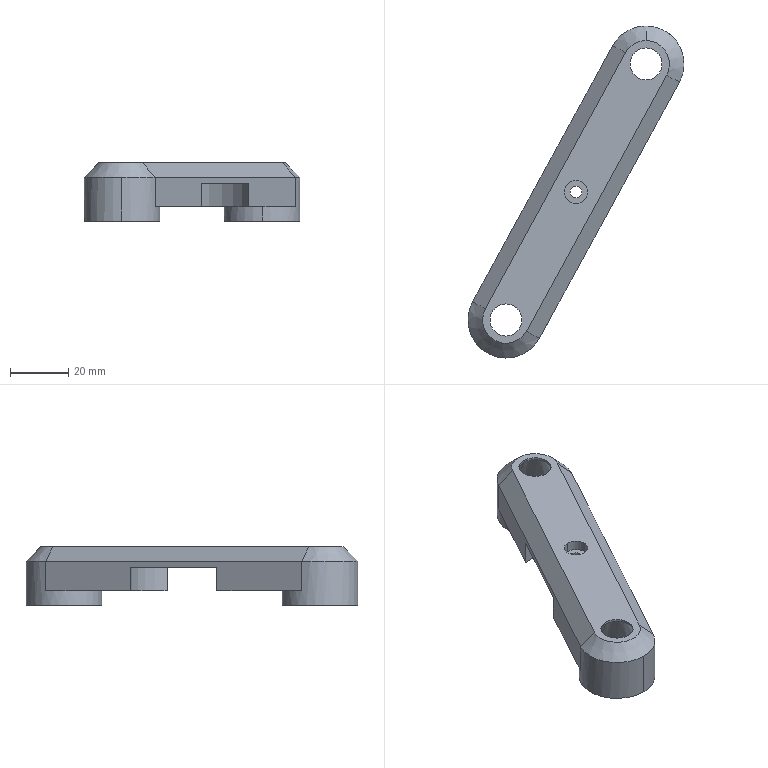Part | SolidWorks | features BaseBody 1 | 1 solid | 39 faces | box 73.991 x 113.732 x 20 mm | volume 29373 mm3 | cylinder 19 | plane 13 | cone 7 | commonest cylinder face diameters 7 x4 11 x4 26 x4 42.5 x3 4 x2 8 x2
STEP:
#1=CARTESIAN_POINT('',(489.266,-50.349,289.248));
#2=VERTEX_POINT('',#1);
#3=CARTESIAN_POINT('',(489.266,-58.349,289.248));
#4=VERTEX_POINT('',#3);
#5=CARTESIAN_POINT('',(489.266,-54.349,289.248));
#6=DIRECTION('',(0.000000004,-0.000000009,1.));
#7=DIRECTION('',(0.,-1.,-0.000000009));
#8=AXIS2_PLACEMENT_3D('',#5,#6,#7);
#9=CIRCLE('',#8,4.);
#10=EDGE_CURVE('',#2,#4,#9,.T.);
#11=ORIENTED_EDGE('',*,*,#10,.F.);
#12=CARTESIAN_POINT('',(489.266,-50.349,292.748));
#13=VERTEX_POINT('',#12);
#14=CARTESIAN_POINT('',(489.266,-50.349,290.998));
#15=DIRECTION('',(0.000000004,-0.000000009,1.));
#16=VECTOR('',#15,1000.);
#17=LINE('',#14,#16);
#18=EDGE_CURVE('',#2,#13,#17,.T.);
#19=ORIENTED_EDGE('',*,*,#18,.T.);
#20=CARTESIAN_POINT('',(489.266,-58.349,292.748));
#21=VERTEX_POINT('',#20);
#22=CARTESIAN_POINT('',(489.266,-54.349,292.748));
#23=DIRECTION('',(0.000000004,-0.000000009,1.));
#24=DIRECTION('',(0.,-1.,-0.000000009));
#25=AXIS2_PLACEMENT_3D('',#22,#23,#24);
#26=CIRCLE('',#25,4.);
#27=EDGE_CURVE('',#13,#21,#26,.T.);
#28=ORIENTED_EDGE('',*,*,#27,.T.);
#29=CARTESIAN_POINT('',(489.266,-58.349,290.998));
#30=DIRECTION('',(0.000000004,-0.000000009,1.));
#31=VECTOR('',#30,1000.);
#32=LINE('',#29,#31);
#33=EDGE_CURVE('',#4,#21,#32,.T.);
#34=ORIENTED_EDGE('',*,*,#33,.F.);
#35=EDGE_LOOP('',(#11,#19,#28,#34));
#36=FACE_OUTER_BOUND('',#35,.T.);
#37=CARTESIAN_POINT('',(489.266,-54.349,290.998));
#38=DIRECTION('',(0.000000004,-0.000000009,1.));
#39=DIRECTION('',(0.,-1.,-0.000000009));
#40=AXIS2_PLACEMENT_3D('',#37,#38,#39);
#41=CYLINDRICAL_SURFACE('',#40,4.);
#42=ADVANCED_FACE('',(#36),#41,.F.);
#43=CARTESIAN_POINT('',(506.243,-6.644,292.748));
#44=VERTEX_POINT('',#43);
#45=CARTESIAN_POINT('',(513.262,-2.483,292.748));
#46=VERTEX_POINT('',#45);
#47=CARTESIAN_POINT('',(513.262,-10.483,292.748));
#48=DIRECTION('',(-0.000000004,0.000000009,-1.));
#49=DIRECTION('',(0.,1.,0.000000009));
#50=AXIS2_PLACEMENT_3D('',#47,#48,#49);
#51=CIRCLE('',#50,8.);
#52=EDGE_CURVE('',#44,#46,#51,.T.);
#53=ORIENTED_EDGE('',*,*,#52,.T.);
#54=CARTESIAN_POINT('',(513.262,2.517,287.748));
#55=VERTEX_POINT('',#54);
#56=CARTESIAN_POINT('',(513.262,2.517,287.748));
#57=DIRECTION('',(-0.000000003,0.7071,-0.7071));
#58=VECTOR('',#57,1000.);
#59=LINE('',#56,#58);
#60=EDGE_CURVE('',#46,#55,#59,.T.);
#61=ORIENTED_EDGE('',*,*,#60,.T.);
#62=CARTESIAN_POINT('',(501.856,-4.244,287.748));
#63=VERTEX_POINT('',#62);
#64=CARTESIAN_POINT('',(513.262,-10.483,287.748));
#65=DIRECTION('',(0.000000004,-0.000000009,1.));
#66=DIRECTION('',(-0.281,0.9597,0.000000009));
#67=AXIS2_PLACEMENT_3D('',#64,#65,#66);
#68=CIRCLE('',#67,13.);
#69=EDGE_CURVE('',#55,#63,#68,.T.);
#70=ORIENTED_EDGE('',*,*,#69,.T.);
#71=CARTESIAN_POINT('',(504.05,-5.444,290.248));
#72=DIRECTION('',(0.6204,-0.3393,0.7071));
#73=VECTOR('',#72,1000.);
#74=LINE('',#71,#73);
#75=EDGE_CURVE('',#63,#44,#74,.T.);
#76=ORIENTED_EDGE('',*,*,#75,.T.);
#77=EDGE_LOOP('',(#53,#61,#70,#76));
#78=FACE_OUTER_BOUND('',#77,.T.);
#79=CARTESIAN_POINT('',(513.262,-10.483,287.748));
#80=DIRECTION('',(-0.000000004,0.000000009,-1.));
#81=DIRECTION('',(0.,1.,0.000000009));
#82=AXIS2_PLACEMENT_3D('',#79,#80,#81);
#83=CONICAL_SURFACE('',#82,13.,0.7854);
#84=ADVANCED_FACE('',(#78),#83,.T.);
#85=CARTESIAN_POINT('',(513.262,-4.983,292.748));
#86=VERTEX_POINT('',#85);
#87=CARTESIAN_POINT('',(513.262,-15.983,292.748));
#88=VERTEX_POINT('',#87);
#89=CARTESIAN_POINT('',(513.262,-10.483,292.748));
#90=DIRECTION('',(0.000000004,-0.000000009,1.));
#91=DIRECTION('',(0.,1.,0.000000009));
#92=AXIS2_PLACEMENT_3D('',#89,#90,#91);
#93=CIRCLE('',#92,5.5);
#94=EDGE_CURVE('',#86,#88,#93,.T.);
#95=ORIENTED_EDGE('',*,*,#94,.T.);
#96=CARTESIAN_POINT('',(513.262,-15.983,291.98));
#97=VERTEX_POINT('',#96);
#98=CARTESIAN_POINT('',(513.262,-15.983,292.364));
#99=DIRECTION('',(-0.000000004,0.000000009,-1.));
#100=VECTOR('',#99,1000.);
#101=LINE('',#98,#100);
#102=EDGE_CURVE('',#88,#97,#101,.T.);
#103=ORIENTED_EDGE('',*,*,#102,.T.);
#104=CARTESIAN_POINT('',(513.262,-4.983,291.98));
#105=VERTEX_POINT('',#104);
#106=CARTESIAN_POINT('',(513.262,-10.483,291.98));
#107=DIRECTION('',(0.000000004,-0.000000009,1.));
#108=DIRECTION('',(0.,1.,0.000000009));
#109=AXIS2_PLACEMENT_3D('',#106,#107,#108);
#110=CIRCLE('',#109,5.5);
#111=EDGE_CURVE('',#105,#97,#110,.T.);
#112=ORIENTED_EDGE('',*,*,#111,.F.);
#113=CARTESIAN_POINT('',(513.262,-4.983,292.364));
#114=DIRECTION('',(-0.000000004,0.000000009,-1.));
#115=VECTOR('',#114,1000.);
#116=LINE('',#113,#115);
#117=EDGE_CURVE('',#86,#105,#116,.T.);
#118=ORIENTED_EDGE('',*,*,#117,.F.);
#119=EDGE_LOOP('',(#95,#103,#112,#118));
#120=FACE_OUTER_BOUND('',#119,.T.);
#121=CARTESIAN_POINT('',(513.262,-10.483,292.364));
#122=DIRECTION('',(-0.000000004,0.000000009,-1.));
#123=DIRECTION('',(0.,1.,0.000000009));
#124=AXIS2_PLACEMENT_3D('',#121,#122,#123);
#125=CYLINDRICAL_SURFACE('',#124,5.5);
#126=ADVANCED_FACE('',(#120),#125,.F.);
#127=CARTESIAN_POINT('',(465.27,-92.715,292.748));
#128=VERTEX_POINT('',#127);
#129=CARTESIAN_POINT('',(465.27,-103.715,292.748));
#130=VERTEX_POINT('',#129);
#131=CARTESIAN_POINT('',(465.27,-98.215,292.748));
#132=DIRECTION('',(0.000000004,-0.000000009,1.));
#133=DIRECTION('',(0.,1.,0.000000009));
#134=AXIS2_PLACEMENT_3D('',#131,#132,#133);
#135=CIRCLE('',#134,5.5);
#136=EDGE_CURVE('',#128,#130,#135,.T.);
#137=ORIENTED_EDGE('',*,*,#136,.T.);
#138=CARTESIAN_POINT('',(465.27,-103.715,291.98));
#139=VERTEX_POINT('',#138);
#140=CARTESIAN_POINT('',(465.27,-103.715,292.364));
#141=DIRECTION('',(-0.000000004,0.000000009,-1.));
#142=VECTOR('',#141,1000.);
#143=LINE('',#140,#142);
#144=EDGE_CURVE('',#130,#139,#143,.T.);
#145=ORIENTED_EDGE('',*,*,#144,.T.);
#146=CARTESIAN_POINT('',(465.27,-92.715,291.98));
#147=VERTEX_POINT('',#146);
#148=CARTESIAN_POINT('',(465.27,-98.215,291.98));
#149=DIRECTION('',(0.000000004,-0.000000009,1.));
#150=DIRECTION('',(0.,1.,0.000000009));
#151=AXIS2_PLACEMENT_3D('',#148,#149,#150);
#152=CIRCLE('',#151,5.5);
#153=EDGE_CURVE('',#147,#139,#152,.T.);
#154=ORIENTED_EDGE('',*,*,#153,.F.);
#155=CARTESIAN_POINT('',(465.27,-92.715,292.364));
#156=DIRECTION('',(-0.000000004,0.000000009,-1.));
#157=VECTOR('',#156,1000.);
#158=LINE('',#155,#157);
#159=EDGE_CURVE('',#128,#147,#158,.T.);
#160=ORIENTED_EDGE('',*,*,#159,.F.);
#161=EDGE_LOOP('',(#137,#145,#154,#160));
#162=FACE_OUTER_BOUND('',#161,.T.);
#163=CARTESIAN_POINT('',(465.27,-98.215,292.364));
#164=DIRECTION('',(-0.000000004,0.000000009,-1.));
#165=DIRECTION('',(0.,1.,0.000000009));
#166=AXIS2_PLACEMENT_3D('',#163,#164,#165);
#167=CYLINDRICAL_SURFACE('',#166,5.5);
#168=ADVANCED_FACE('',(#162),#167,.F.);
#169=CARTESIAN_POINT('',(465.27,-111.215,272.748));
#170=VERTEX_POINT('',#169);
#171=CARTESIAN_POINT('',(465.27,-85.215,272.748));
#172=VERTEX_POINT('',#171);
#173=CARTESIAN_POINT('',(465.27,-98.215,272.748));
#174=DIRECTION('',(0.000000004,-0.000000009,1.));
#175=DIRECTION('',(0.,-1.,-0.000000009));
#176=AXIS2_PLACEMENT_3D('',#173,#174,#175);
#177=CIRCLE('',#176,13.);
#178=EDGE_CURVE('',#170,#172,#177,.T.);
#179=ORIENTED_EDGE('',*,*,#178,.T.);
#180=CARTESIAN_POINT('',(465.27,-85.215,277.748));
#181=VERTEX_POINT('',#180);
#182=CARTESIAN_POINT('',(465.27,-85.215,292.748));
#183=DIRECTION('',(0.000000004,-0.000000009,1.));
#184=VECTOR('',#183,1000.);
#185=LINE('',#182,#184);
#186=EDGE_CURVE('',#172,#181,#185,.T.);
#187=ORIENTED_EDGE('',*,*,#186,.T.);
#188=CARTESIAN_POINT('',(476.675,-104.454,277.748));
#189=VERTEX_POINT('',#188);
#190=CARTESIAN_POINT('',(465.27,-98.215,277.748));
#191=DIRECTION('',(-0.000000004,0.000000009,-1.));
#192=DIRECTION('',(0.,-1.,-0.000000009));
#193=AXIS2_PLACEMENT_3D('',#190,#191,#192);
#194=CIRCLE('',#193,13.);
#195=EDGE_CURVE('',#181,#189,#194,.T.);
#196=ORIENTED_EDGE('',*,*,#195,.T.);
#197=CARTESIAN_POINT('',(476.675,-104.454,287.748));
#198=VERTEX_POINT('',#197);
#199=CARTESIAN_POINT('',(476.675,-104.454,292.748));
#200=DIRECTION('',(0.000000004,-0.000000009,1.));
#201=VECTOR('',#200,1000.);
#202=LINE('',#199,#201);
#203=EDGE_CURVE('',#189,#198,#202,.T.);
#204=ORIENTED_EDGE('',*,*,#203,.T.);
#205=CARTESIAN_POINT('',(465.27,-111.215,287.748));
#206=VERTEX_POINT('',#205);
#207=CARTESIAN_POINT('',(465.27,-98.215,287.748));
#208=DIRECTION('',(0.000000004,-0.000000009,1.));
#209=DIRECTION('',(-0.9597,-0.281,0.000000001));
#210=AXIS2_PLACEMENT_3D('',#207,#208,#209);
#211=CIRCLE('',#210,13.);
#212=EDGE_CURVE('',#206,#198,#211,.T.);
#213=ORIENTED_EDGE('',*,*,#212,.F.);
#214=CARTESIAN_POINT('',(465.27,-111.215,292.748));
#215=DIRECTION('',(0.000000004,-0.000000009,1.));
#216=VECTOR('',#215,1000.);
#217=LINE('',#214,#216);
#218=EDGE_CURVE('',#170,#206,#217,.T.);
#219=ORIENTED_EDGE('',*,*,#218,.F.);
#220=EDGE_LOOP('',(#179,#187,#196,#204,#213,#219));
#221=FACE_OUTER_BOUND('',#220,.T.);
#222=CARTESIAN_POINT('',(465.27,-98.215,292.748));
#223=DIRECTION('',(0.000000004,-0.000000009,1.));
#224=DIRECTION('',(0.,-1.,-0.000000009));
#225=AXIS2_PLACEMENT_3D('',#222,#223,#224);
#226=CYLINDRICAL_SURFACE('',#225,13.);
#227=ADVANCED_FACE('',(#221),#226,.T.);
#228=CARTESIAN_POINT('',(513.262,-23.483,272.748));
#229=VERTEX_POINT('',#228);
#230=CARTESIAN_POINT('',(513.262,2.517,272.748));
#231=VERTEX_POINT('',#230);
#232=CARTESIAN_POINT('',(513.262,-10.483,272.748));
#233=DIRECTION('',(0.000000004,-0.000000009,1.));
#234=DIRECTION('',(0.,-1.,-0.000000009));
#235=AXIS2_PLACEMENT_3D('',#232,#233,#234);
#236=CIRCLE('',#235,13.);
#237=EDGE_CURVE('',#229,#231,#236,.T.);
#238=ORIENTED_EDGE('',*,*,#237,.T.);
#239=CARTESIAN_POINT('',(513.262,2.517,292.748));
#240=DIRECTION('',(0.000000004,-0.000000009,1.));
#241=VECTOR('',#240,1000.);
#242=LINE('',#239,#241);
#243=EDGE_CURVE('',#231,#55,#242,.T.);
#244=ORIENTED_EDGE('',*,*,#243,.T.);
#245=CARTESIAN_POINT('',(524.667,-16.722,287.748));
#246=VERTEX_POINT('',#245);
#247=CARTESIAN_POINT('',(513.262,-10.483,287.748));
#248=DIRECTION('',(0.000000004,-0.000000009,1.));
#249=DIRECTION('',(-0.281,0.9597,0.000000009));
#250=AXIS2_PLACEMENT_3D('',#247,#248,#249);
#251=CIRCLE('',#250,13.);
#252=EDGE_CURVE('',#246,#55,#251,.T.);
#253=ORIENTED_EDGE('',*,*,#252,.F.);
#254=CARTESIAN_POINT('',(524.667,-16.722,277.748));
#255=VERTEX_POINT('',#254);
#256=CARTESIAN_POINT('',(524.667,-16.722,292.748));
#257=DIRECTION('',(0.000000007,-0.000000004,1.));
#258=VECTOR('',#257,1000.);
#259=LINE('',#256,#258);
#260=EDGE_CURVE('',#255,#246,#259,.T.);
#261=ORIENTED_EDGE('',*,*,#260,.F.);
#262=CARTESIAN_POINT('',(513.262,-23.483,277.748));
#263=VERTEX_POINT('',#262);
#264=CARTESIAN_POINT('',(513.262,-10.483,277.748));
#265=DIRECTION('',(-0.000000004,0.000000009,-1.));
#266=DIRECTION('',(0.,-1.,-0.000000009));
#267=AXIS2_PLACEMENT_3D('',#264,#265,#266);
#268=CIRCLE('',#267,13.);
#269=EDGE_CURVE('',#255,#263,#268,.T.);
#270=ORIENTED_EDGE('',*,*,#269,.T.);
#271=CARTESIAN_POINT('',(513.262,-23.483,292.748));
#272=DIRECTION('',(0.000000004,-0.000000009,1.));
#273=VECTOR('',#272,1000.);
#274=LINE('',#271,#273);
#275=EDGE_CURVE('',#229,#263,#274,.T.);
#276=ORIENTED_EDGE('',*,*,#275,.F.);
#277=EDGE_LOOP('',(#238,#244,#253,#261,#270,#276));
#278=FACE_OUTER_BOUND('',#277,.T.);
#279=CARTESIAN_POINT('',(513.262,-10.483,292.748));
#280=DIRECTION('',(0.000000004,-0.000000009,1.));
#281=DIRECTION('',(0.,-1.,-0.000000009));
#282=AXIS2_PLACEMENT_3D('',#279,#280,#281);
#283=CYLINDRICAL_SURFACE('',#282,13.);
#284=ADVANCED_FACE('',(#278),#283,.T.);
#285=ORIENTED_EDGE('',*,*,#111,.T.);
#286=CARTESIAN_POINT('',(513.262,-22.983,272.748));
#287=VERTEX_POINT('',#286);
#288=CARTESIAN_POINT('',(513.262,-22.983,272.748));
#289=DIRECTION('',(-0.000000004,-0.342,-0.9397));
#290=VECTOR('',#289,1000.);
#291=LINE('',#288,#290);
#292=EDGE_CURVE('',#97,#287,#291,.T.);
#293=ORIENTED_EDGE('',*,*,#292,.T.);
#294=CARTESIAN_POINT('',(513.262,2.017,272.748));
#295=VERTEX_POINT('',#294);
#296=CARTESIAN_POINT('',(513.262,-10.483,272.748));
#297=DIRECTION('',(0.000000004,-0.000000009,1.));
#298=DIRECTION('',(0.,1.,0.000000009));
#299=AXIS2_PLACEMENT_3D('',#296,#297,#298);
#300=CIRCLE('',#299,12.5);
#301=EDGE_CURVE('',#295,#287,#300,.T.);
#302=ORIENTED_EDGE('',*,*,#301,.F.);
#303=CARTESIAN_POINT('',(513.262,2.017,272.748));
#304=DIRECTION('',(-0.000000004,0.342,-0.9397));
#305=VECTOR('',#304,1000.);
#306=LINE('',#303,#305);
#307=EDGE_CURVE('',#105,#295,#306,.T.);
#308=ORIENTED_EDGE('',*,*,#307,.F.);
#309=EDGE_LOOP('',(#285,#293,#302,#308));
#310=FACE_OUTER_BOUND('',#309,.T.);
#311=CARTESIAN_POINT('',(513.262,-10.483,272.748));
#312=DIRECTION('',(-0.000000004,0.000000009,-1.));
#313=DIRECTION('',(0.,1.,0.000000009));
#314=AXIS2_PLACEMENT_3D('',#311,#312,#313);
#315=CONICAL_SURFACE('',#314,12.5,0.3491);
#316=ADVANCED_FACE('',(#310),#315,.F.);
#317=ORIENTED_EDGE('',*,*,#153,.T.);
#318=CARTESIAN_POINT('',(465.27,-110.715,272.748));
#319=VERTEX_POINT('',#318);
#320=CARTESIAN_POINT('',(465.27,-110.715,272.748));
#321=DIRECTION('',(-0.000000004,-0.342,-0.9397));
#322=VECTOR('',#321,1000.);
#323=LINE('',#320,#322);
#324=EDGE_CURVE('',#139,#319,#323,.T.);
#325=ORIENTED_EDGE('',*,*,#324,.T.);
#326=CARTESIAN_POINT('',(465.27,-85.715,272.748));
#327=VERTEX_POINT('',#326);
#328=CARTESIAN_POINT('',(465.27,-98.215,272.748));
#329=DIRECTION('',(0.000000004,-0.000000009,1.));
#330=DIRECTION('',(0.,1.,0.000000009));
#331=AXIS2_PLACEMENT_3D('',#328,#329,#330);
#332=CIRCLE('',#331,12.5);
#333=EDGE_CURVE('',#327,#319,#332,.T.);
#334=ORIENTED_EDGE('',*,*,#333,.F.);
#335=CARTESIAN_POINT('',(465.27,-85.715,272.748));
#336=DIRECTION('',(-0.000000004,0.342,-0.9397));
#337=VECTOR('',#336,1000.);
#338=LINE('',#335,#337);
#339=EDGE_CURVE('',#147,#327,#338,.T.);
#340=ORIENTED_EDGE('',*,*,#339,.F.);
#341=EDGE_LOOP('',(#317,#325,#334,#340));
#342=FACE_OUTER_BOUND('',#341,.T.);
#343=CARTESIAN_POINT('',(465.27,-98.215,272.748));
#344=DIRECTION('',(-0.000000004,0.000000009,-1.));
#345=DIRECTION('',(0.,1.,0.000000009));
#346=AXIS2_PLACEMENT_3D('',#343,#344,#345);
#347=CONICAL_SURFACE('',#346,12.5,0.3491);
#348=ADVANCED_FACE('',(#342),#347,.F.);
#349=CARTESIAN_POINT('',(489.266,-52.349,285.748));
#350=VERTEX_POINT('',#349);
#351=CARTESIAN_POINT('',(489.266,-56.349,285.748));
#352=VERTEX_POINT('',#351);
#353=CARTESIAN_POINT('',(489.266,-54.349,285.748));
#354=DIRECTION('',(0.000000004,-0.000000009,1.));
#355=DIRECTION('',(0.,-1.,-0.000000009));
#356=AXIS2_PLACEMENT_3D('',#353,#354,#355);
#357=CIRCLE('',#356,2.);
#358=EDGE_CURVE('',#350,#352,#357,.T.);
#359=ORIENTED_EDGE('',*,*,#358,.F.);
#360=CARTESIAN_POINT('',(489.266,-52.349,289.248));
#361=VERTEX_POINT('',#360);
#362=CARTESIAN_POINT('',(489.266,-52.349,285.998));
#363=DIRECTION('',(0.000000004,-0.000000009,1.));
#364=VECTOR('',#363,1000.);
#365=LINE('',#362,#364);
#366=EDGE_CURVE('',#350,#361,#365,.T.);
#367=ORIENTED_EDGE('',*,*,#366,.T.);
#368=CARTESIAN_POINT('',(489.266,-56.349,289.248));
#369=VERTEX_POINT('',#368);
#370=CARTESIAN_POINT('',(489.266,-54.349,289.248));
#371=DIRECTION('',(0.000000004,-0.000000009,1.));
#372=DIRECTION('',(0.,-1.,-0.000000009));
#373=AXIS2_PLACEMENT_3D('',#370,#371,#372);
#374=CIRCLE('',#373,2.);
#375=EDGE_CURVE('',#361,#369,#374,.T.);
#376=ORIENTED_EDGE('',*,*,#375,.T.);
#377=CARTESIAN_POINT('',(489.266,-56.349,285.998));
#378=DIRECTION('',(0.000000004,-0.000000009,1.));
#379=VECTOR('',#378,1000.);
#380=LINE('',#377,#379);
#381=EDGE_CURVE('',#352,#369,#380,.T.);
#382=ORIENTED_EDGE('',*,*,#381,.F.);
#383=EDGE_LOOP('',(#359,#367,#376,#382));
#384=FACE_OUTER_BOUND('',#383,.T.);
#385=CARTESIAN_POINT('',(489.266,-54.349,285.998));
#386=DIRECTION('',(0.000000004,-0.000000009,1.));
#387=DIRECTION('',(0.,-1.,-0.000000009));
#388=AXIS2_PLACEMENT_3D('',#385,#386,#387);
#389=CYLINDRICAL_SURFACE('',#388,2.);
#390=ADVANCED_FACE('',(#384),#389,.F.);
#391=CARTESIAN_POINT('',(492.604,-75.335,277.748));
#392=VERTEX_POINT('',#391);
#393=CARTESIAN_POINT('',(489.266,-75.599,277.748));
#394=VERTEX_POINT('',#393);
#395=CARTESIAN_POINT('',(489.266,-54.349,277.748));
#396=DIRECTION('',(-0.000000004,0.000000009,-1.));
#397=DIRECTION('',(0.,-1.,-0.000000009));
#398=AXIS2_PLACEMENT_3D('',#395,#396,#397);
#399=CIRCLE('',#398,21.25);
#400=EDGE_CURVE('',#392,#394,#399,.T.);
#401=ORIENTED_EDGE('',*,*,#400,.T.);
#402=CARTESIAN_POINT('',(489.266,-75.599,285.748));
#403=VERTEX_POINT('',#402);
#404=CARTESIAN_POINT('',(489.266,-75.599,271.501));
#405=DIRECTION('',(0.000000004,-0.000000009,1.));
#406=VECTOR('',#405,1000.);
#407=LINE('',#404,#406);
#408=EDGE_CURVE('',#394,#403,#407,.T.);
#409=ORIENTED_EDGE('',*,*,#408,.T.);
#410=CARTESIAN_POINT('',(492.604,-75.335,285.748));
#411=VERTEX_POINT('',#410);
#412=CARTESIAN_POINT('',(489.266,-54.349,285.748));
#413=DIRECTION('',(0.000000004,-0.000000009,1.));
#414=DIRECTION('',(0.,-1.,-0.000000009));
#415=AXIS2_PLACEMENT_3D('',#412,#413,#414);
#416=CIRCLE('',#415,21.25);
#417=EDGE_CURVE('',#403,#411,#416,.T.);
#418=ORIENTED_EDGE('',*,*,#417,.T.);
#419=CARTESIAN_POINT('',(492.604,-75.335,292.748));
#420=DIRECTION('',(0.000000007,-0.000000004,1.));
#421=VECTOR('',#420,1000.);
#422=LINE('',#419,#421);
#423=EDGE_CURVE('',#392,#411,#422,.T.);
#424=ORIENTED_EDGE('',*,*,#423,.F.);
#425=EDGE_LOOP('',(#401,#409,#418,#424));
#426=FACE_OUTER_BOUND('',#425,.T.);
#427=CARTESIAN_POINT('',(489.266,-54.349,271.501));
#428=DIRECTION('',(0.000000004,-0.000000009,1.));
#429=DIRECTION('',(0.,-1.,-0.000000009));
#430=AXIS2_PLACEMENT_3D('',#427,#428,#429);
#431=CYLINDRICAL_SURFACE('',#430,21.25);
#432=ADVANCED_FACE('',(#426),#431,.F.);
#433=CARTESIAN_POINT('',(476.308,-81.537,285.666));
#434=VERTEX_POINT('',#433);
#435=CARTESIAN_POINT('',(476.308,-74.537,285.666));
#436=VERTEX_POINT('',#435);
#437=CARTESIAN_POINT('',(476.308,-78.037,285.666));
#438=DIRECTION('',(-0.000000004,0.000000009,-1.));
#439=DIRECTION('',(0.,1.,0.000000009));
#440=AXIS2_PLACEMENT_3D('',#437,#438,#439);
#441=CIRCLE('',#440,3.5);
#442=EDGE_CURVE('',#434,#436,#441,.T.);
#443=ORIENTED_EDGE('',*,*,#442,.F.);
#444=CARTESIAN_POINT('',(476.308,-81.537,277.748));
#445=VERTEX_POINT('',#444);
#446=CARTESIAN_POINT('',(476.308,-81.537,260.666));
#447=DIRECTION('',(-0.000000004,0.000000009,-1.));
#448=VECTOR('',#447,1000.);
#449=LINE('',#446,#448);
#450=EDGE_CURVE('',#434,#445,#449,.T.);
#451=ORIENTED_EDGE('',*,*,#450,.T.);
#452=CARTESIAN_POINT('',(476.308,-74.537,277.748));
#453=VERTEX_POINT('',#452);
#454=CARTESIAN_POINT('',(476.308,-78.037,277.748));
#455=DIRECTION('',(-0.000000004,0.000000009,-1.));
#456=DIRECTION('',(0.,1.,0.000000009));
#457=AXIS2_PLACEMENT_3D('',#454,#455,#456);
#458=CIRCLE('',#457,3.5);
#459=EDGE_CURVE('',#445,#453,#458,.T.);
#460=ORIENTED_EDGE('',*,*,#459,.T.);
#461=CARTESIAN_POINT('',(476.308,-74.537,260.666));
#462=DIRECTION('',(-0.000000004,0.000000009,-1.));
#463=VECTOR('',#462,1000.);
#464=LINE('',#461,#463);
#465=EDGE_CURVE('',#436,#453,#464,.T.);
#466=ORIENTED_EDGE('',*,*,#465,.F.);
#467=EDGE_LOOP('',(#443,#451,#460,#466));
#468=FACE_OUTER_BOUND('',#467,.T.);
#469=CARTESIAN_POINT('',(476.308,-78.037,260.666));
#470=DIRECTION('',(-0.000000004,0.000000009,-1.));
#471=DIRECTION('',(0.,1.,0.000000009));
#472=AXIS2_PLACEMENT_3D('',#469,#470,#471);
#473=CYLINDRICAL_SURFACE('',#472,3.5);
#474=ADVANCED_FACE('',(#468),#473,.F.);
#475=CARTESIAN_POINT('',(502.224,-34.162,285.666));
#476=VERTEX_POINT('',#475);
#477=CARTESIAN_POINT('',(502.224,-27.162,285.666));
#478=VERTEX_POINT('',#477);
#479=CARTESIAN_POINT('',(502.224,-30.662,285.666));
#480=DIRECTION('',(-0.000000004,0.000000009,-1.));
#481=DIRECTION('',(0.,1.,0.000000009));
#482=AXIS2_PLACEMENT_3D('',#479,#480,#481);
#483=CIRCLE('',#482,3.5);
#484=EDGE_CURVE('',#476,#478,#483,.T.);
#485=ORIENTED_EDGE('',*,*,#484,.F.);
#486=CARTESIAN_POINT('',(502.224,-34.162,277.748));
#487=VERTEX_POINT('',#486);
#488=CARTESIAN_POINT('',(502.224,-34.162,260.666));
#489=DIRECTION('',(-0.000000004,0.000000009,-1.));
#490=VECTOR('',#489,1000.);
#491=LINE('',#488,#490);
#492=EDGE_CURVE('',#476,#487,#491,.T.);
#493=ORIENTED_EDGE('',*,*,#492,.T.);
#494=CARTESIAN_POINT('',(502.224,-27.162,277.748));
#495=VERTEX_POINT('',#494);
#496=CARTESIAN_POINT('',(502.224,-30.662,277.748));
#497=DIRECTION('',(-0.000000004,0.000000009,-1.));
#498=DIRECTION('',(0.,1.,0.000000009));
#499=AXIS2_PLACEMENT_3D('',#496,#497,#498);
#500=CIRCLE('',#499,3.5);
#501=EDGE_CURVE('',#487,#495,#500,.T.);
#502=ORIENTED_EDGE('',*,*,#501,.T.);
#503=CARTESIAN_POINT('',(502.224,-27.162,260.666));
#504=DIRECTION('',(-0.000000004,0.000000009,-1.));
#505=VECTOR('',#504,1000.);
#506=LINE('',#503,#505);
#507=EDGE_CURVE('',#478,#495,#506,.T.);
#508=ORIENTED_EDGE('',*,*,#507,.F.);
#509=EDGE_LOOP('',(#485,#493,#502,#508));
#510=FACE_OUTER_BOUND('',#509,.T.);
#511=CARTESIAN_POINT('',(502.224,-30.662,260.666));
#512=DIRECTION('',(-0.000000004,0.000000009,-1.));
#513=DIRECTION('',(0.,1.,0.000000009));
#514=AXIS2_PLACEMENT_3D('',#511,#512,#513);
#515=CYLINDRICAL_SURFACE('',#514,3.5);
#516=ADVANCED_FACE('',(#510),#515,.F.);
#517=CARTESIAN_POINT('',(489.266,-54.349,292.748));
#518=DIRECTION('',(0.000000004,-0.000000009,1.));
#519=DIRECTION('',(0.,-1.,-0.000000009));
#520=AXIS2_PLACEMENT_3D('',#517,#518,#519);
#521=CIRCLE('',#520,4.);
#522=EDGE_CURVE('',#21,#13,#521,.T.);
#523=ORIENTED_EDGE('',*,*,#522,.F.);
#524=ORIENTED_EDGE('',*,*,#27,.F.);
#525=EDGE_LOOP('',(#523,#524));
#526=FACE_BOUND('',#525,.T.);
#527=CARTESIAN_POINT('',(520.28,-14.323,292.748));
#528=VERTEX_POINT('',#527);
#529=CARTESIAN_POINT('',(472.289,-102.054,292.748));
#530=VERTEX_POINT('',#529);
#531=CARTESIAN_POINT('',(520.28,-14.323,292.748));
#532=DIRECTION('',(-0.4799,-0.8773,-0.000000006));
#533=VECTOR('',#532,1000.);
#534=LINE('',#531,#533);
#535=EDGE_CURVE('',#528,#530,#534,.T.);
#536=ORIENTED_EDGE('',*,*,#535,.F.);
#537=CARTESIAN_POINT('',(513.262,-10.483,292.748));
#538=DIRECTION('',(-0.000000004,0.000000009,-1.));
#539=DIRECTION('',(0.,1.,0.000000009));
#540=AXIS2_PLACEMENT_3D('',#537,#538,#539);
#541=CIRCLE('',#540,8.);
#542=EDGE_CURVE('',#46,#528,#541,.T.);
#543=ORIENTED_EDGE('',*,*,#542,.F.);
#544=ORIENTED_EDGE('',*,*,#52,.F.);
#545=CARTESIAN_POINT('',(458.252,-94.376,292.748));
#546=VERTEX_POINT('',#545);
#547=CARTESIAN_POINT('',(458.252,-94.376,292.748));
#548=DIRECTION('',(0.4799,0.8773,0.000000006));
#549=VECTOR('',#548,1000.);
#550=LINE('',#547,#549);
#551=EDGE_CURVE('',#546,#44,#550,.T.);
#552=ORIENTED_EDGE('',*,*,#551,.F.);
#553=CARTESIAN_POINT('',(465.27,-98.215,292.748));
#554=DIRECTION('',(-0.000000004,0.000000009,-1.));
#555=DIRECTION('',(0.,1.,0.000000009));
#556=AXIS2_PLACEMENT_3D('',#553,#554,#555);
#557=CIRCLE('',#556,8.);
#558=EDGE_CURVE('',#530,#546,#557,.T.);
#559=ORIENTED_EDGE('',*,*,#558,.F.);
#560=EDGE_LOOP('',(#536,#543,#544,#552,#559));
#561=FACE_OUTER_BOUND('',#560,.T.);
#562=ORIENTED_EDGE('',*,*,#94,.F.);
#563=CARTESIAN_POINT('',(513.262,-10.483,292.748));
#564=DIRECTION('',(0.000000004,-0.000000009,1.));
#565=DIRECTION('',(0.,1.,0.000000009));
#566=AXIS2_PLACEMENT_3D('',#563,#564,#565);
#567=CIRCLE('',#566,5.5);
#568=EDGE_CURVE('',#88,#86,#567,.T.);
#569=ORIENTED_EDGE('',*,*,#568,.F.);
#570=EDGE_LOOP('',(#562,#569));
#571=FACE_BOUND('',#570,.T.);
#572=ORIENTED_EDGE('',*,*,#136,.F.);
#573=CARTESIAN_POINT('',(465.27,-98.215,292.748));
#574=DIRECTION('',(0.000000004,-0.000000009,1.));
#575=DIRECTION('',(0.,1.,0.000000009));
#576=AXIS2_PLACEMENT_3D('',#573,#574,#575);
#577=CIRCLE('',#576,5.5);
#578=EDGE_CURVE('',#130,#128,#577,.T.);
#579=ORIENTED_EDGE('',*,*,#578,.F.);
#580=EDGE_LOOP('',(#572,#579));
#581=FACE_BOUND('',#580,.T.);
#582=CARTESIAN_POINT('',(489.266,-54.349,292.748));
#583=DIRECTION('',(-0.000000004,0.000000009,-1.));
#584=DIRECTION('',(0.,1.,0.000000009));
#585=AXIS2_PLACEMENT_3D('',#582,#583,#584);
#586=PLANE('',#585);
#587=ADVANCED_FACE('',(#526,#561,#571,#581),#586,.F.);
#588=ORIENTED_EDGE('',*,*,#18,.F.);
#589=CARTESIAN_POINT('',(489.266,-54.349,289.248));
#590=DIRECTION('',(0.000000004,-0.000000009,1.));
#591=DIRECTION('',(0.,-1.,-0.000000009));
#592=AXIS2_PLACEMENT_3D('',#589,#590,#591);
#593=CIRCLE('',#592,4.);
#594=EDGE_CURVE('',#4,#2,#593,.T.);
#595=ORIENTED_EDGE('',*,*,#594,.F.);
#596=ORIENTED_EDGE('',*,*,#33,.T.);
#597=ORIENTED_EDGE('',*,*,#522,.T.);
#598=EDGE_LOOP('',(#588,#595,#596,#597));
#599=FACE_OUTER_BOUND('',#598,.T.);
#600=CARTESIAN_POINT('',(489.266,-54.349,290.998));
#601=DIRECTION('',(0.000000004,-0.000000009,1.));
#602=DIRECTION('',(0.,-1.,-0.000000009));
#603=AXIS2_PLACEMENT_3D('',#600,#601,#602);
#604=CYLINDRICAL_SURFACE('',#603,4.);
#605=ADVANCED_FACE('',(#599),#604,.F.);
#606=CARTESIAN_POINT('',(474.482,-103.254,290.248));
#607=DIRECTION('',(-0.6204,0.3393,0.7071));
#608=VECTOR('',#607,1000.);
#609=LINE('',#606,#608);
#610=EDGE_CURVE('',#198,#530,#609,.T.);
#611=ORIENTED_EDGE('',*,*,#610,.T.);
#612=ORIENTED_EDGE('',*,*,#558,.T.);
#613=CARTESIAN_POINT('',(453.865,-91.976,287.748));
#614=VERTEX_POINT('',#613);
#615=CARTESIAN_POINT('',(453.865,-91.976,287.748));
#616=DIRECTION('',(0.6204,-0.3393,0.7071));
#617=VECTOR('',#616,1000.);
#618=LINE('',#615,#617);
#619=EDGE_CURVE('',#614,#546,#618,.T.);
#620=ORIENTED_EDGE('',*,*,#619,.F.);
#621=CARTESIAN_POINT('',(465.27,-98.215,287.748));
#622=DIRECTION('',(0.000000004,-0.000000009,1.));
#623=DIRECTION('',(-0.9597,-0.281,0.000000001));
#624=AXIS2_PLACEMENT_3D('',#621,#622,#623);
#625=CIRCLE('',#624,13.);
#626=EDGE_CURVE('',#614,#206,#625,.T.);
#627=ORIENTED_EDGE('',*,*,#626,.T.);
#628=ORIENTED_EDGE('',*,*,#212,.T.);
#629=EDGE_LOOP('',(#611,#612,#620,#627,#628));
#630=FACE_OUTER_BOUND('',#629,.T.);
#631=CARTESIAN_POINT('',(465.27,-98.215,287.748));
#632=DIRECTION('',(-0.000000004,0.000000009,-1.));
#633=DIRECTION('',(0.,1.,0.000000009));
#634=AXIS2_PLACEMENT_3D('',#631,#632,#633);
#635=CONICAL_SURFACE('',#634,13.,0.7854);
#636=ADVANCED_FACE('',(#630),#635,.T.);
#637=CARTESIAN_POINT('',(524.667,-16.722,287.748));
#638=DIRECTION('',(-0.6204,0.3393,0.7071));
#639=VECTOR('',#638,1000.);
#640=LINE('',#637,#639);
#641=EDGE_CURVE('',#246,#528,#640,.T.);
#642=ORIENTED_EDGE('',*,*,#641,.T.);
#643=ORIENTED_EDGE('',*,*,#535,.T.);
#644=ORIENTED_EDGE('',*,*,#610,.F.);
#645=CARTESIAN_POINT('',(476.675,-104.454,287.748));
#646=DIRECTION('',(0.4799,0.8773,0.000000006));
#647=VECTOR('',#646,1000.);
#648=LINE('',#645,#647);
#649=EDGE_CURVE('',#198,#246,#648,.T.);
#650=ORIENTED_EDGE('',*,*,#649,.T.);
#651=EDGE_LOOP('',(#642,#643,#644,#650));
#652=FACE_OUTER_BOUND('',#651,.T.);
#653=CARTESIAN_POINT('',(483.36,-87.024,290.248));
#654=DIRECTION('',(0.6204,-0.3393,0.7071));
#655=DIRECTION('',(0.7517,0.,-0.6595));
#656=AXIS2_PLACEMENT_3D('',#653,#654,#655);
#657=PLANE('',#656);
#658=ADVANCED_FACE('',(#652),#657,.T.);
#659=ORIENTED_EDGE('',*,*,#60,.F.);
#660=ORIENTED_EDGE('',*,*,#542,.T.);
#661=ORIENTED_EDGE('',*,*,#641,.F.);
#662=ORIENTED_EDGE('',*,*,#252,.T.);
#663=EDGE_LOOP('',(#659,#660,#661,#662));
#664=FACE_OUTER_BOUND('',#663,.T.);
#665=CARTESIAN_POINT('',(513.262,-10.483,287.748));
#666=DIRECTION('',(-0.000000004,0.000000009,-1.));
#667=DIRECTION('',(0.,1.,0.000000009));
#668=AXIS2_PLACEMENT_3D('',#665,#666,#667);
#669=CONICAL_SURFACE('',#668,13.,0.7854);
#670=ADVANCED_FACE('',(#664),#669,.T.);
#671=ORIENTED_EDGE('',*,*,#75,.F.);
#672=CARTESIAN_POINT('',(501.856,-4.244,287.748));
#673=DIRECTION('',(-0.4799,-0.8773,-0.000000006));
#674=VECTOR('',#673,1000.);
#675=LINE('',#672,#674);
#676=EDGE_CURVE('',#63,#614,#675,.T.);
#677=ORIENTED_EDGE('',*,*,#676,.T.);
#678=ORIENTED_EDGE('',*,*,#619,.T.);
#679=ORIENTED_EDGE('',*,*,#551,.T.);
#680=EDGE_LOOP('',(#671,#677,#678,#679));
#681=FACE_OUTER_BOUND('',#680,.T.);
#682=CARTESIAN_POINT('',(495.171,-21.675,290.248));
#683=DIRECTION('',(-0.6204,0.3393,0.7071));
#684=DIRECTION('',(0.7517,0.,0.6595));
#685=AXIS2_PLACEMENT_3D('',#682,#683,#684);
#686=PLANE('',#685);
#687=ADVANCED_FACE('',(#681),#686,.T.);
#688=ORIENTED_EDGE('',*,*,#102,.F.);
#689=ORIENTED_EDGE('',*,*,#568,.T.);
#690=ORIENTED_EDGE('',*,*,#117,.T.);
#691=CARTESIAN_POINT('',(513.262,-10.483,291.98));
#692=DIRECTION('',(0.000000004,-0.000000009,1.));
#693=DIRECTION('',(0.,1.,0.000000009));
#694=AXIS2_PLACEMENT_3D('',#691,#692,#693);
#695=CIRCLE('',#694,5.5);
#696=EDGE_CURVE('',#97,#105,#695,.T.);
#697=ORIENTED_EDGE('',*,*,#696,.F.);
#698=EDGE_LOOP('',(#688,#689,#690,#697));
#699=FACE_OUTER_BOUND('',#698,.T.);
#700=CARTESIAN_POINT('',(513.262,-10.483,292.364));
#701=DIRECTION('',(-0.000000004,0.000000009,-1.));
#702=DIRECTION('',(0.,1.,0.000000009));
#703=AXIS2_PLACEMENT_3D('',#700,#701,#702);
#704=CYLINDRICAL_SURFACE('',#703,5.5);
#705=ADVANCED_FACE('',(#699),#704,.F.);
#706=ORIENTED_EDGE('',*,*,#144,.F.);
#707=ORIENTED_EDGE('',*,*,#578,.T.);
#708=ORIENTED_EDGE('',*,*,#159,.T.);
#709=CARTESIAN_POINT('',(465.27,-98.215,291.98));
#710=DIRECTION('',(0.000000004,-0.000000009,1.));
#711=DIRECTION('',(0.,1.,0.000000009));
#712=AXIS2_PLACEMENT_3D('',#709,#710,#711);
#713=CIRCLE('',#712,5.5);
#714=EDGE_CURVE('',#139,#147,#713,.T.);
#715=ORIENTED_EDGE('',*,*,#714,.F.);
#716=EDGE_LOOP('',(#706,#707,#708,#715));
#717=FACE_OUTER_BOUND('',#716,.T.);
#718=CARTESIAN_POINT('',(465.27,-98.215,292.364));
#719=DIRECTION('',(-0.000000004,0.000000009,-1.));
#720=DIRECTION('',(0.,1.,0.000000009));
#721=AXIS2_PLACEMENT_3D('',#718,#719,#720);
#722=CYLINDRICAL_SURFACE('',#721,5.5);
#723=ADVANCED_FACE('',(#717),#722,.F.);
#724=ORIENTED_EDGE('',*,*,#594,.T.);
#725=ORIENTED_EDGE('',*,*,#10,.T.);
#726=EDGE_LOOP('',(#724,#725));
#727=FACE_OUTER_BOUND('',#726,.T.);
#728=CARTESIAN_POINT('',(489.266,-54.349,289.248));
#729=DIRECTION('',(0.000000004,-0.000000009,1.));
#730=DIRECTION('',(0.,-1.,-0.000000009));
#731=AXIS2_PLACEMENT_3D('',#728,#729,#730);
#732=CIRCLE('',#731,2.);
#733=EDGE_CURVE('',#369,#361,#732,.T.);
#734=ORIENTED_EDGE('',*,*,#733,.F.);
#735=ORIENTED_EDGE('',*,*,#375,.F.);
#736=EDGE_LOOP('',(#734,#735));
#737=FACE_BOUND('',#736,.T.);
#738=CARTESIAN_POINT('',(487.826,-56.981,289.248));
#739=DIRECTION('',(-0.000000004,0.000000009,-1.));
#740=DIRECTION('',(0.,1.,0.000000009));
#741=AXIS2_PLACEMENT_3D('',#738,#739,#740);
#742=PLANE('',#741);
#743=ADVANCED_FACE('',(#727,#737),#742,.F.);
#744=ORIENTED_EDGE('',*,*,#186,.F.);
#745=CARTESIAN_POINT('',(465.27,-98.215,272.748));
#746=DIRECTION('',(0.000000004,-0.000000009,1.));
#747=DIRECTION('',(0.,-1.,-0.000000009));
#748=AXIS2_PLACEMENT_3D('',#745,#746,#747);
#749=CIRCLE('',#748,13.);
#750=EDGE_CURVE('',#172,#170,#749,.T.);
#751=ORIENTED_EDGE('',*,*,#750,.T.);
#752=ORIENTED_EDGE('',*,*,#218,.T.);
#753=ORIENTED_EDGE('',*,*,#626,.F.);
#754=CARTESIAN_POINT('',(453.865,-91.976,277.748));
#755=VERTEX_POINT('',#754);
#756=CARTESIAN_POINT('',(453.865,-91.976,292.748));
#757=DIRECTION('',(0.000000007,-0.000000004,1.));
#758=VECTOR('',#757,1000.);
#759=LINE('',#756,#758);
#760=EDGE_CURVE('',#755,#614,#759,.T.);
#761=ORIENTED_EDGE('',*,*,#760,.F.);
#762=CARTESIAN_POINT('',(465.27,-98.215,277.748));
#763=DIRECTION('',(-0.000000004,0.000000009,-1.));
#764=DIRECTION('',(0.,-1.,-0.000000009));
#765=AXIS2_PLACEMENT_3D('',#762,#763,#764);
#766=CIRCLE('',#765,13.);
#767=EDGE_CURVE('',#755,#181,#766,.T.);
#768=ORIENTED_EDGE('',*,*,#767,.T.);
#769=EDGE_LOOP('',(#744,#751,#752,#753,#761,#768));
#770=FACE_OUTER_BOUND('',#769,.T.);
#771=CARTESIAN_POINT('',(465.27,-98.215,292.748));
#772=DIRECTION('',(0.000000004,-0.000000009,1.));
#773=DIRECTION('',(0.,-1.,-0.000000009));
#774=AXIS2_PLACEMENT_3D('',#771,#772,#773);
#775=CYLINDRICAL_SURFACE('',#774,13.);
#776=ADVANCED_FACE('',(#770),#775,.T.);
#777=ORIENTED_EDGE('',*,*,#649,.F.);
#778=ORIENTED_EDGE('',*,*,#203,.F.);
#779=CARTESIAN_POINT('',(470.436,-115.859,277.748));
#780=DIRECTION('',(0.4799,0.8773,0.));
#781=VECTOR('',#780,1000.);
#782=LINE('',#779,#781);
#783=EDGE_CURVE('',#189,#392,#782,.T.);
#784=ORIENTED_EDGE('',*,*,#783,.T.);
#785=ORIENTED_EDGE('',*,*,#423,.T.);
#786=CARTESIAN_POINT('',(508.738,-45.841,285.748));
#787=VERTEX_POINT('',#786);
#788=CARTESIAN_POINT('',(470.436,-115.859,285.748));
#789=DIRECTION('',(0.4799,0.8773,0.));
#790=VECTOR('',#789,1000.);
#791=LINE('',#788,#790);
#792=EDGE_CURVE('',#411,#787,#791,.T.);
#793=ORIENTED_EDGE('',*,*,#792,.T.);
#794=CARTESIAN_POINT('',(508.738,-45.841,277.748));
#795=VERTEX_POINT('',#794);
#796=CARTESIAN_POINT('',(508.738,-45.841,292.748));
#797=DIRECTION('',(-0.000000007,0.000000004,-1.));
#798=VECTOR('',#797,1000.);
#799=LINE('',#796,#798);
#800=EDGE_CURVE('',#787,#795,#799,.T.);
#801=ORIENTED_EDGE('',*,*,#800,.T.);
#802=CARTESIAN_POINT('',(470.436,-115.859,277.748));
#803=DIRECTION('',(0.4799,0.8773,0.));
#804=VECTOR('',#803,1000.);
#805=LINE('',#802,#804);
#806=EDGE_CURVE('',#795,#255,#805,.T.);
#807=ORIENTED_EDGE('',*,*,#806,.T.);
#808=ORIENTED_EDGE('',*,*,#260,.T.);
#809=EDGE_LOOP('',(#777,#778,#784,#785,#793,#801,#807,#808));
#810=FACE_OUTER_BOUND('',#809,.T.);
#811=CARTESIAN_POINT('',(470.436,-115.859,292.748));
#812=DIRECTION('',(0.8773,-0.4799,-0.000000008));
#813=DIRECTION('',(0.4799,0.8773,0.));
#814=AXIS2_PLACEMENT_3D('',#811,#812,#813);
#815=PLANE('',#814);
#816=ADVANCED_FACE('',(#810),#815,.T.);
#817=ORIENTED_EDGE('',*,*,#243,.F.);
#818=CARTESIAN_POINT('',(513.262,-10.483,272.748));
#819=DIRECTION('',(0.000000004,-0.000000009,1.));
#820=DIRECTION('',(0.,-1.,-0.000000009));
#821=AXIS2_PLACEMENT_3D('',#818,#819,#820);
#822=CIRCLE('',#821,13.);
#823=EDGE_CURVE('',#231,#229,#822,.T.);
#824=ORIENTED_EDGE('',*,*,#823,.T.);
#825=ORIENTED_EDGE('',*,*,#275,.T.);
#826=CARTESIAN_POINT('',(501.856,-4.244,277.748));
#827=VERTEX_POINT('',#826);
#828=CARTESIAN_POINT('',(513.262,-10.483,277.748));
#829=DIRECTION('',(-0.000000004,0.000000009,-1.));
#830=DIRECTION('',(0.,-1.,-0.000000009));
#831=AXIS2_PLACEMENT_3D('',#828,#829,#830);
#832=CIRCLE('',#831,13.);
#833=EDGE_CURVE('',#263,#827,#832,.T.);
#834=ORIENTED_EDGE('',*,*,#833,.T.);
#835=CARTESIAN_POINT('',(501.856,-4.244,292.748));
#836=DIRECTION('',(0.000000004,-0.000000009,1.));
#837=VECTOR('',#836,1000.);
#838=LINE('',#835,#837);
#839=EDGE_CURVE('',#827,#63,#838,.T.);
#840=ORIENTED_EDGE('',*,*,#839,.T.);
#841=ORIENTED_EDGE('',*,*,#69,.F.);
#842=EDGE_LOOP('',(#817,#824,#825,#834,#840,#841));
#843=FACE_OUTER_BOUND('',#842,.T.);
#844=CARTESIAN_POINT('',(513.262,-10.483,292.748));
#845=DIRECTION('',(0.000000004,-0.000000009,1.));
#846=DIRECTION('',(0.,-1.,-0.000000009));
#847=AXIS2_PLACEMENT_3D('',#844,#845,#846);
#848=CYLINDRICAL_SURFACE('',#847,13.);
#849=ADVANCED_FACE('',(#843),#848,.T.);
#850=CARTESIAN_POINT('',(485.928,-33.363,285.748));
#851=VERTEX_POINT('',#850);
#852=CARTESIAN_POINT('',(469.794,-62.858,285.748));
#853=VERTEX_POINT('',#852);
#854=CARTESIAN_POINT('',(508.095,7.161,285.748));
#855=DIRECTION('',(-0.4799,-0.8773,0.));
#856=VECTOR('',#855,1000.);
#857=LINE('',#854,#856);
#858=EDGE_CURVE('',#851,#853,#857,.T.);
#859=ORIENTED_EDGE('',*,*,#858,.T.);
#860=CARTESIAN_POINT('',(469.794,-62.858,277.748));
#861=VERTEX_POINT('',#860);
#862=CARTESIAN_POINT('',(469.794,-62.858,292.748));
#863=DIRECTION('',(-0.000000007,0.000000004,-1.));
#864=VECTOR('',#863,1000.);
#865=LINE('',#862,#864);
#866=EDGE_CURVE('',#853,#861,#865,.T.);
#867=ORIENTED_EDGE('',*,*,#866,.T.);
#868=CARTESIAN_POINT('',(508.095,7.161,277.748));
#869=DIRECTION('',(-0.4799,-0.8773,0.));
#870=VECTOR('',#869,1000.);
#871=LINE('',#868,#870);
#872=EDGE_CURVE('',#861,#755,#871,.T.);
#873=ORIENTED_EDGE('',*,*,#872,.T.);
#874=ORIENTED_EDGE('',*,*,#760,.T.);
#875=ORIENTED_EDGE('',*,*,#676,.F.);
#876=ORIENTED_EDGE('',*,*,#839,.F.);
#877=CARTESIAN_POINT('',(485.928,-33.363,277.748));
#878=VERTEX_POINT('',#877);
#879=CARTESIAN_POINT('',(508.095,7.161,277.748));
#880=DIRECTION('',(-0.4799,-0.8773,0.));
#881=VECTOR('',#880,1000.);
#882=LINE('',#879,#881);
#883=EDGE_CURVE('',#827,#878,#882,.T.);
#884=ORIENTED_EDGE('',*,*,#883,.T.);
#885=CARTESIAN_POINT('',(485.928,-33.363,292.748));
#886=DIRECTION('',(0.000000007,-0.000000004,1.));
#887=VECTOR('',#886,1000.);
#888=LINE('',#885,#887);
#889=EDGE_CURVE('',#878,#851,#888,.T.);
#890=ORIENTED_EDGE('',*,*,#889,.T.);
#891=EDGE_LOOP('',(#859,#867,#873,#874,#875,#876,#884,#890));
#892=FACE_OUTER_BOUND('',#891,.T.);
#893=CARTESIAN_POINT('',(508.095,7.161,292.748));
#894=DIRECTION('',(-0.8773,0.4799,0.000000008));
#895=DIRECTION('',(-0.4799,-0.8773,0.));
#896=AXIS2_PLACEMENT_3D('',#893,#894,#895);
#897=PLANE('',#896);
#898=ADVANCED_FACE('',(#892),#897,.T.);
#899=ORIENTED_EDGE('',*,*,#292,.F.);
#900=ORIENTED_EDGE('',*,*,#696,.T.);
#901=ORIENTED_EDGE('',*,*,#307,.T.);
#902=CARTESIAN_POINT('',(513.262,-10.483,272.748));
#903=DIRECTION('',(0.000000004,-0.000000009,1.));
#904=DIRECTION('',(0.,1.,0.000000009));
#905=AXIS2_PLACEMENT_3D('',#902,#903,#904);
#906=CIRCLE('',#905,12.5);
#907=EDGE_CURVE('',#287,#295,#906,.T.);
#908=ORIENTED_EDGE('',*,*,#907,.F.);
#909=EDGE_LOOP('',(#899,#900,#901,#908));
#910=FACE_OUTER_BOUND('',#909,.T.);
#911=CARTESIAN_POINT('',(513.262,-10.483,272.748));
#912=DIRECTION('',(-0.000000004,0.000000009,-1.));
#913=DIRECTION('',(0.,1.,0.000000009));
#914=AXIS2_PLACEMENT_3D('',#911,#912,#913);
#915=CONICAL_SURFACE('',#914,12.5,0.3491);
#916=ADVANCED_FACE('',(#910),#915,.F.);
#917=ORIENTED_EDGE('',*,*,#324,.F.);
#918=ORIENTED_EDGE('',*,*,#714,.T.);
#919=ORIENTED_EDGE('',*,*,#339,.T.);
#920=CARTESIAN_POINT('',(465.27,-98.215,272.748));
#921=DIRECTION('',(0.000000004,-0.000000009,1.));
#922=DIRECTION('',(0.,1.,0.000000009));
#923=AXIS2_PLACEMENT_3D('',#920,#921,#922);
#924=CIRCLE('',#923,12.5);
#925=EDGE_CURVE('',#319,#327,#924,.T.);
#926=ORIENTED_EDGE('',*,*,#925,.F.);
#927=EDGE_LOOP('',(#917,#918,#919,#926));
#928=FACE_OUTER_BOUND('',#927,.T.);
#929=CARTESIAN_POINT('',(465.27,-98.215,272.748));
#930=DIRECTION('',(-0.000000004,0.000000009,-1.));
#931=DIRECTION('',(0.,1.,0.000000009));
#932=AXIS2_PLACEMENT_3D('',#929,#930,#931);
#933=CONICAL_SURFACE('',#932,12.5,0.3491);
#934=ADVANCED_FACE('',(#928),#933,.F.);
#935=ORIENTED_EDGE('',*,*,#366,.F.);
#936=CARTESIAN_POINT('',(489.266,-54.349,285.748));
#937=DIRECTION('',(0.000000004,-0.000000009,1.));
#938=DIRECTION('',(0.,-1.,-0.000000009));
#939=AXIS2_PLACEMENT_3D('',#936,#937,#938);
#940=CIRCLE('',#939,2.);
#941=EDGE_CURVE('',#352,#350,#940,.T.);
#942=ORIENTED_EDGE('',*,*,#941,.F.);
#943=ORIENTED_EDGE('',*,*,#381,.T.);
#944=ORIENTED_EDGE('',*,*,#733,.T.);
#945=EDGE_LOOP('',(#935,#942,#943,#944));
#946=FACE_OUTER_BOUND('',#945,.T.);
#947=CARTESIAN_POINT('',(489.266,-54.349,285.998));
#948=DIRECTION('',(0.000000004,-0.000000009,1.));
#949=DIRECTION('',(0.,-1.,-0.000000009));
#950=AXIS2_PLACEMENT_3D('',#947,#948,#949);
#951=CYLINDRICAL_SURFACE('',#950,2.);
#952=ADVANCED_FACE('',(#946),#951,.F.);
#953=ORIENTED_EDGE('',*,*,#783,.F.);
#954=ORIENTED_EDGE('',*,*,#195,.F.);
#955=ORIENTED_EDGE('',*,*,#767,.F.);
#956=ORIENTED_EDGE('',*,*,#872,.F.);
#957=CARTESIAN_POINT('',(489.266,-54.349,277.748));
#958=DIRECTION('',(-0.000000004,0.000000009,-1.));
#959=DIRECTION('',(0.,-1.,-0.000000009));
#960=AXIS2_PLACEMENT_3D('',#957,#958,#959);
#961=CIRCLE('',#960,21.25);
#962=EDGE_CURVE('',#394,#861,#961,.T.);
#963=ORIENTED_EDGE('',*,*,#962,.F.);
#964=ORIENTED_EDGE('',*,*,#400,.F.);
#965=EDGE_LOOP('',(#953,#954,#955,#956,#963,#964));
#966=FACE_OUTER_BOUND('',#965,.T.);
#967=CARTESIAN_POINT('',(476.308,-78.037,277.748));
#968=DIRECTION('',(-0.000000004,0.000000009,-1.));
#969=DIRECTION('',(0.,1.,0.000000009));
#970=AXIS2_PLACEMENT_3D('',#967,#968,#969);
#971=CIRCLE('',#970,3.5);
#972=EDGE_CURVE('',#453,#445,#971,.T.);
#973=ORIENTED_EDGE('',*,*,#972,.F.);
#974=ORIENTED_EDGE('',*,*,#459,.F.);
#975=EDGE_LOOP('',(#973,#974));
#976=FACE_BOUND('',#975,.T.);
#977=CARTESIAN_POINT('',(489.266,-54.349,277.748));
#978=DIRECTION('',(0.000000004,-0.000000009,1.));
#979=DIRECTION('',(0.,-1.,-0.000000009));
#980=AXIS2_PLACEMENT_3D('',#977,#978,#979);
#981=PLANE('',#980);
#982=ADVANCED_FACE('',(#966,#976),#981,.F.);
#983=ORIENTED_EDGE('',*,*,#333,.T.);
#984=ORIENTED_EDGE('',*,*,#925,.T.);
#985=EDGE_LOOP('',(#983,#984));
#986=FACE_BOUND('',#985,.T.);
#987=ORIENTED_EDGE('',*,*,#178,.F.);
#988=ORIENTED_EDGE('',*,*,#750,.F.);
#989=EDGE_LOOP('',(#987,#988));
#990=FACE_OUTER_BOUND('',#989,.T.);
#991=CARTESIAN_POINT('',(489.266,-54.349,272.748));
#992=DIRECTION('',(-0.000000004,0.000000009,-1.));
#993=DIRECTION('',(0.,1.,0.000000009));
#994=AXIS2_PLACEMENT_3D('',#991,#992,#993);
#995=PLANE('',#994);
#996=ADVANCED_FACE('',(#986,#990),#995,.T.);
#997=ORIENTED_EDGE('',*,*,#883,.F.);
#998=ORIENTED_EDGE('',*,*,#833,.F.);
#999=ORIENTED_EDGE('',*,*,#269,.F.);
#1000=ORIENTED_EDGE('',*,*,#806,.F.);
#1001=CARTESIAN_POINT('',(489.266,-54.349,277.748));
#1002=DIRECTION('',(-0.000000004,0.000000009,-1.));
#1003=DIRECTION('',(0.,-1.,-0.000000009));
#1004=AXIS2_PLACEMENT_3D('',#1001,#1002,#1003);
#1005=CIRCLE('',#1004,21.25);
#1006=EDGE_CURVE('',#878,#795,#1005,.T.);
#1007=ORIENTED_EDGE('',*,*,#1006,.F.);
#1008=EDGE_LOOP('',(#997,#998,#999,#1000,#1007));
#1009=FACE_OUTER_BOUND('',#1008,.T.);
#1010=CARTESIAN_POINT('',(502.224,-30.662,277.748));
#1011=DIRECTION('',(-0.000000004,0.000000009,-1.));
#1012=DIRECTION('',(0.,1.,0.000000009));
#1013=AXIS2_PLACEMENT_3D('',#1010,#1011,#1012);
#1014=CIRCLE('',#1013,3.5);
#1015=EDGE_CURVE('',#495,#487,#1014,.T.);
#1016=ORIENTED_EDGE('',*,*,#1015,.F.);
#1017=ORIENTED_EDGE('',*,*,#501,.F.);
#1018=EDGE_LOOP('',(#1016,#1017));
#1019=FACE_BOUND('',#1018,.T.);
#1020=CARTESIAN_POINT('',(489.266,-54.349,277.748));
#1021=DIRECTION('',(0.000000004,-0.000000009,1.));
#1022=DIRECTION('',(0.,-1.,-0.000000009));
#1023=AXIS2_PLACEMENT_3D('',#1020,#1021,#1022);
#1024=PLANE('',#1023);
#1025=ADVANCED_FACE('',(#1009,#1019),#1024,.F.);
#1026=ORIENTED_EDGE('',*,*,#1006,.T.);
#1027=ORIENTED_EDGE('',*,*,#800,.F.);
#1028=CARTESIAN_POINT('',(489.266,-54.349,285.748));
#1029=DIRECTION('',(-0.000000004,0.000000009,-1.));
#1030=DIRECTION('',(0.,-1.,-0.000000009));
#1031=AXIS2_PLACEMENT_3D('',#1028,#1029,#1030);
#1032=CIRCLE('',#1031,21.25);
#1033=EDGE_CURVE('',#851,#787,#1032,.T.);
#1034=ORIENTED_EDGE('',*,*,#1033,.F.);
#1035=ORIENTED_EDGE('',*,*,#889,.F.);
#1036=EDGE_LOOP('',(#1026,#1027,#1034,#1035));
#1037=FACE_OUTER_BOUND('',#1036,.T.);
#1038=CARTESIAN_POINT('',(489.266,-54.349,271.501));
#1039=DIRECTION('',(0.000000004,-0.000000009,1.));
#1040=DIRECTION('',(0.,-1.,-0.000000009));
#1041=AXIS2_PLACEMENT_3D('',#1038,#1039,#1040);
#1042=CYLINDRICAL_SURFACE('',#1041,21.25);
#1043=ADVANCED_FACE('',(#1037),#1042,.F.);
#1044=CARTESIAN_POINT('',(489.266,-54.349,285.748));
#1045=DIRECTION('',(0.000000004,-0.000000009,1.));
#1046=DIRECTION('',(0.,-1.,-0.000000009));
#1047=AXIS2_PLACEMENT_3D('',#1044,#1045,#1046);
#1048=CIRCLE('',#1047,21.25);
#1049=EDGE_CURVE('',#853,#403,#1048,.T.);
#1050=ORIENTED_EDGE('',*,*,#1049,.F.);
#1051=ORIENTED_EDGE('',*,*,#858,.F.);
#1052=ORIENTED_EDGE('',*,*,#1033,.T.);
#1053=ORIENTED_EDGE('',*,*,#792,.F.);
#1054=ORIENTED_EDGE('',*,*,#417,.F.);
#1055=EDGE_LOOP('',(#1050,#1051,#1052,#1053,#1054));
#1056=FACE_OUTER_BOUND('',#1055,.T.);
#1057=ORIENTED_EDGE('',*,*,#941,.T.);
#1058=ORIENTED_EDGE('',*,*,#358,.T.);
#1059=EDGE_LOOP('',(#1057,#1058));
#1060=FACE_BOUND('',#1059,.T.);
#1061=CARTESIAN_POINT('',(489.266,-54.349,285.748));
#1062=DIRECTION('',(0.000000004,-0.000000009,1.));
#1063=DIRECTION('',(0.,-1.,-0.000000009));
#1064=AXIS2_PLACEMENT_3D('',#1061,#1062,#1063);
#1065=PLANE('',#1064);
#1066=ADVANCED_FACE('',(#1056,#1060),#1065,.F.);
#1067=ORIENTED_EDGE('',*,*,#408,.F.);
#1068=ORIENTED_EDGE('',*,*,#962,.T.);
#1069=ORIENTED_EDGE('',*,*,#866,.F.);
#1070=ORIENTED_EDGE('',*,*,#1049,.T.);
#1071=EDGE_LOOP('',(#1067,#1068,#1069,#1070));
#1072=FACE_OUTER_BOUND('',#1071,.T.);
#1073=CARTESIAN_POINT('',(489.266,-54.349,271.501));
#1074=DIRECTION('',(0.000000004,-0.000000009,1.));
#1075=DIRECTION('',(0.,-1.,-0.000000009));
#1076=AXIS2_PLACEMENT_3D('',#1073,#1074,#1075);
#1077=CYLINDRICAL_SURFACE('',#1076,21.25);
#1078=ADVANCED_FACE('',(#1072),#1077,.F.);
#1079=ORIENTED_EDGE('',*,*,#301,.T.);
#1080=ORIENTED_EDGE('',*,*,#907,.T.);
#1081=EDGE_LOOP('',(#1079,#1080));
#1082=FACE_BOUND('',#1081,.T.);
#1083=ORIENTED_EDGE('',*,*,#237,.F.);
#1084=ORIENTED_EDGE('',*,*,#823,.F.);
#1085=EDGE_LOOP('',(#1083,#1084));
#1086=FACE_OUTER_BOUND('',#1085,.T.);
#1087=CARTESIAN_POINT('',(489.266,-54.349,272.748));
#1088=DIRECTION('',(-0.000000004,0.000000009,-1.));
#1089=DIRECTION('',(0.,1.,0.000000009));
#1090=AXIS2_PLACEMENT_3D('',#1087,#1088,#1089);
#1091=PLANE('',#1090);
#1092=ADVANCED_FACE('',(#1082,#1086),#1091,.T.);
#1093=ORIENTED_EDGE('',*,*,#450,.F.);
#1094=CARTESIAN_POINT('',(476.308,-78.037,285.666));
#1095=DIRECTION('',(-0.000000004,0.000000009,-1.));
#1096=DIRECTION('',(0.,1.,0.000000009));
#1097=AXIS2_PLACEMENT_3D('',#1094,#1095,#1096);
#1098=CIRCLE('',#1097,3.5);
#1099=EDGE_CURVE('',#436,#434,#1098,.T.);
#1100=ORIENTED_EDGE('',*,*,#1099,.F.);
#1101=ORIENTED_EDGE('',*,*,#465,.T.);
#1102=ORIENTED_EDGE('',*,*,#972,.T.);
#1103=EDGE_LOOP('',(#1093,#1100,#1101,#1102));
#1104=FACE_OUTER_BOUND('',#1103,.T.);
#1105=CARTESIAN_POINT('',(476.308,-78.037,260.666));
#1106=DIRECTION('',(-0.000000004,0.000000009,-1.));
#1107=DIRECTION('',(0.,1.,0.000000009));
#1108=AXIS2_PLACEMENT_3D('',#1105,#1106,#1107);
#1109=CYLINDRICAL_SURFACE('',#1108,3.5);
#1110=ADVANCED_FACE('',(#1104),#1109,.F.);
#1111=ORIENTED_EDGE('',*,*,#492,.F.);
#1112=CARTESIAN_POINT('',(502.224,-30.662,285.666));
#1113=DIRECTION('',(-0.000000004,0.000000009,-1.));
#1114=DIRECTION('',(0.,1.,0.000000009));
#1115=AXIS2_PLACEMENT_3D('',#1112,#1113,#1114);
#1116=CIRCLE('',#1115,3.5);
#1117=EDGE_CURVE('',#478,#476,#1116,.T.);
#1118=ORIENTED_EDGE('',*,*,#1117,.F.);
#1119=ORIENTED_EDGE('',*,*,#507,.T.);
#1120=ORIENTED_EDGE('',*,*,#1015,.T.);
#1121=EDGE_LOOP('',(#1111,#1118,#1119,#1120));
#1122=FACE_OUTER_BOUND('',#1121,.T.);
#1123=CARTESIAN_POINT('',(502.224,-30.662,260.666));
#1124=DIRECTION('',(-0.000000004,0.000000009,-1.));
#1125=DIRECTION('',(0.,1.,0.000000009));
#1126=AXIS2_PLACEMENT_3D('',#1123,#1124,#1125);
#1127=CYLINDRICAL_SURFACE('',#1126,3.5);
#1128=ADVANCED_FACE('',(#1122),#1127,.F.);
#1129=ORIENTED_EDGE('',*,*,#1099,.T.);
#1130=ORIENTED_EDGE('',*,*,#442,.T.);
#1131=EDGE_LOOP('',(#1129,#1130));
#1132=FACE_OUTER_BOUND('',#1131,.T.);
#1133=CARTESIAN_POINT('',(476.308,-78.037,285.666));
#1134=DIRECTION('',(0.000000004,-0.000000009,1.));
#1135=DIRECTION('',(0.,-1.,-0.000000009));
#1136=AXIS2_PLACEMENT_3D('',#1133,#1134,#1135);
#1137=PLANE('',#1136);
#1138=ADVANCED_FACE('',(#1132),#1137,.F.);
#1139=ORIENTED_EDGE('',*,*,#1117,.T.);
#1140=ORIENTED_EDGE('',*,*,#484,.T.);
#1141=EDGE_LOOP('',(#1139,#1140));
#1142=FACE_OUTER_BOUND('',#1141,.T.);
#1143=CARTESIAN_POINT('',(502.224,-30.662,285.666));
#1144=DIRECTION('',(0.000000004,-0.000000009,1.));
#1145=DIRECTION('',(0.,-1.,-0.000000009));
#1146=AXIS2_PLACEMENT_3D('',#1143,#1144,#1145);
#1147=PLANE('',#1146);
#1148=ADVANCED_FACE('',(#1142),#1147,.F.);
#1149=CLOSED_SHELL('',(#42,#84,#126,#168,#227,#284,#316,#348,#390,#432,#474,#516,#587,#605,#636,#658,#670,#687,#705,#723,#743,#776,#816,#849,#898,#916,#934,#952,#982,#996,#1025,#1043,#1066,#1078,#1092,#1110,#1128,#1138,#1148));
#1150=MANIFOLD_SOLID_BREP('',#1149);
#1151=CARTESIAN_POINT('',(0.,0.,0.));
#1152=DIRECTION('',(0.,0.,1.));
#1153=DIRECTION('',(1.,0.,0.));
#1154=AXIS2_PLACEMENT_3D('',#1151,#1152,#1153);
#1155=(LENGTH_UNIT()NAMED_UNIT(*)SI_UNIT(.MILLI.,.METRE.));
#1156=UNCERTAINTY_MEASURE_WITH_UNIT(LENGTH_MEASURE(0.00001),#1155,'','');
#1157=(NAMED_UNIT(*)PLANE_ANGLE_UNIT()SI_UNIT($,.RADIAN.));
#1158=(NAMED_UNIT(*)SI_UNIT($,.STERADIAN.)SOLID_ANGLE_UNIT());
#1159=(GEOMETRIC_REPRESENTATION_CONTEXT(3)GLOBAL_UNCERTAINTY_ASSIGNED_CONTEXT((#1156))GLOBAL_UNIT_ASSIGNED_CONTEXT((#1155,#1157,#1158))REPRESENTATION_CONTEXT('',''));
#1160=ADVANCED_BREP_SHAPE_REPRESENTATION('',(#1150,#1154),#1159);